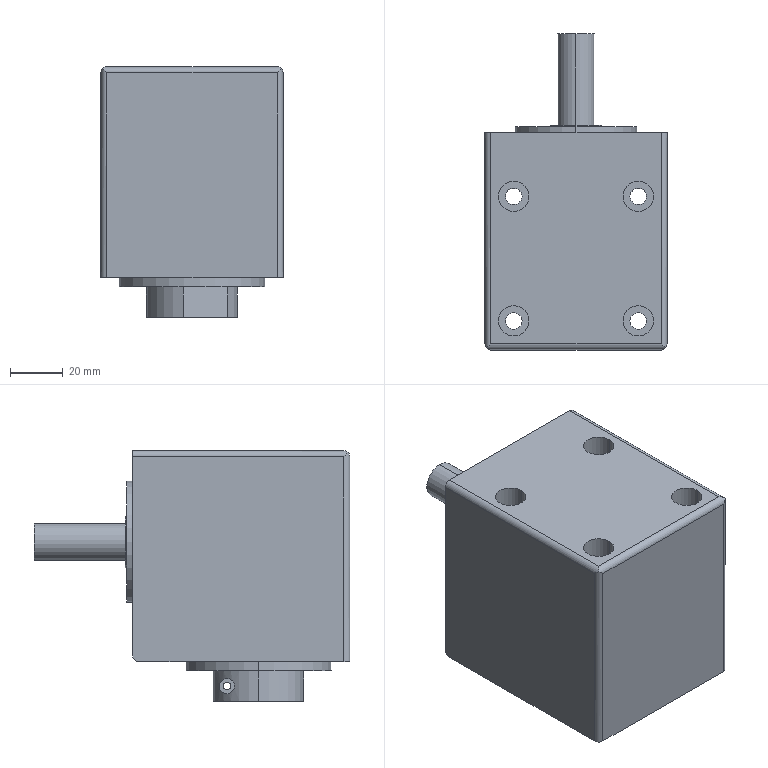Part | SolidWorks | features BaseBody 1 | 1 solid | 81 faces | box 69.231 x 120 x 95.192 mm | volume 467345 mm3 | cylinder 49 | plane 24 | cone 8 | commonest cylinder face diameters 4.77 x8 6.346 x8 11.538 x8 4.615 x6 2.885 x4 13.846 x4